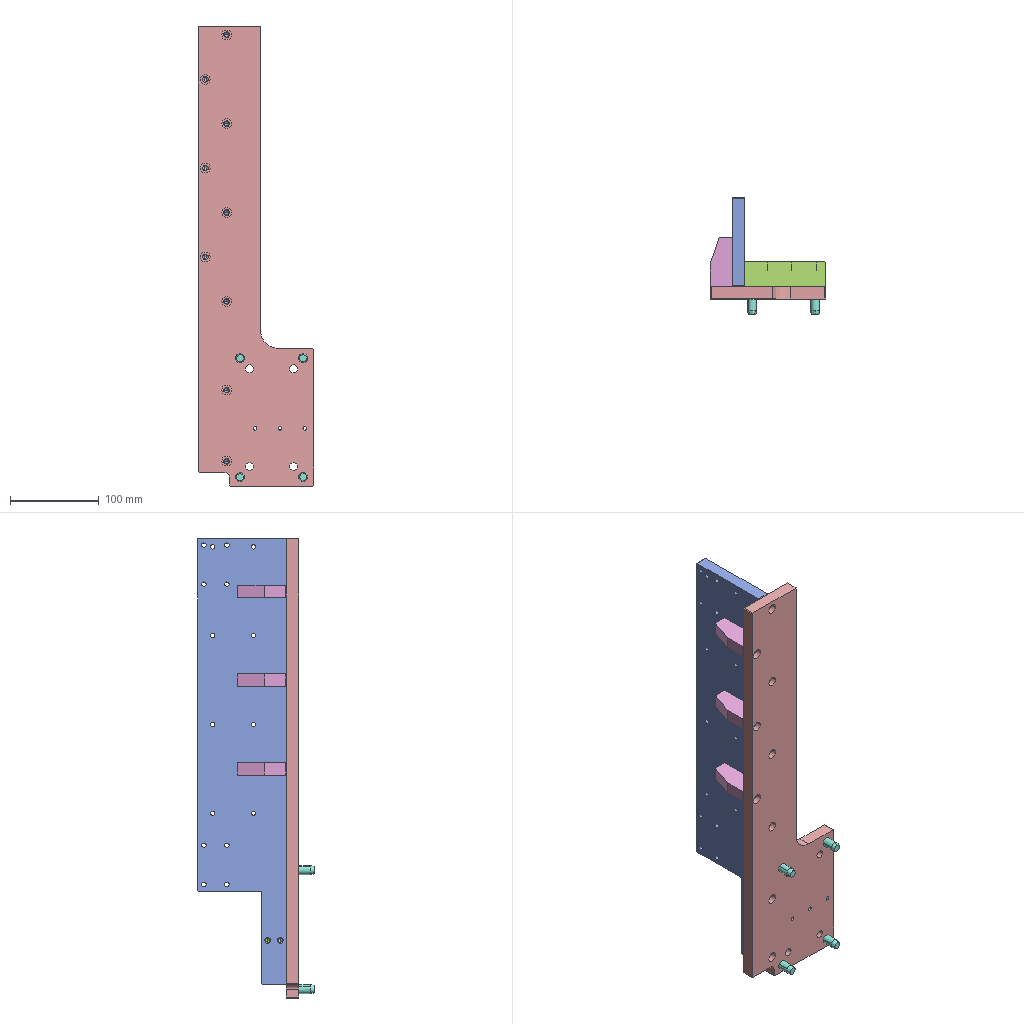Assembly | SolidWorks | 11 different items | 16 placed | box 130 x 132 x 518 mm
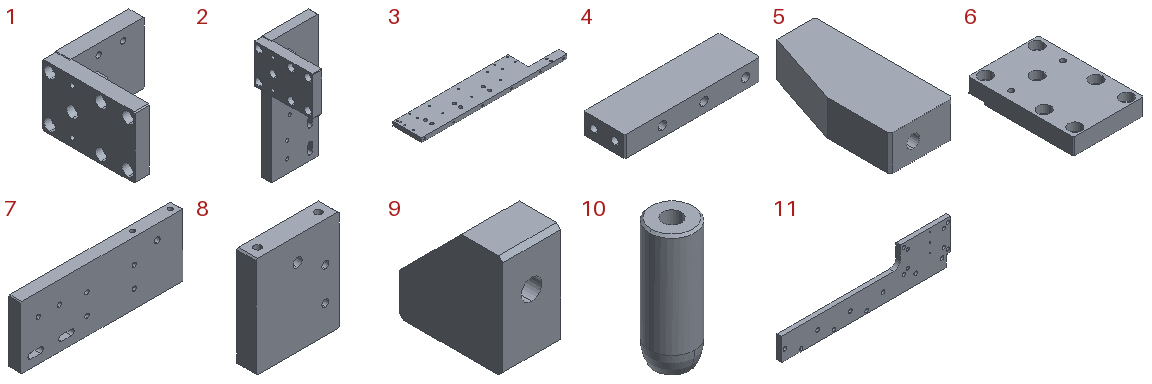Parts list (item | name | quantity | size | volume | features):
1 | (subassembly) | x1 | 85 x 90 x 60 mm | 133215 mm3 | -
2 | (subassembly) | x1 | 85 x 90 x 189 mm | 260889 mm3 | -
3 | - | x1 | 503 x 100 x 14 mm | 585787 mm3 | features HoleWzd 5, Chamfer 1, Extrusion 1, ICE 1
4 | - | x1 | 91 x 28 x 14 mm | 31396 mm3 | features HoleWzd 2, Chamfer 1, Extrusion 1
5 | - | x3 | 25 x 55 x 14 mm | 16216 mm3 | features HoleWzd 2, Chamfer 1, Extrusion 1
6 | - | x1 | 60 x 90 x 14 mm | 67395 mm3 | features HoleWzd 2, Chamfer 1, Extrusion 1, ICE 1
7 | - | x1 | 189 x 14 x 73 mm | 186915 mm3 | features HoleWzd 5, Chamfer 1, Extrusion 1
8 | - | x1 | 60 x 14 x 73 mm | 59241 mm3 | features HoleWzd 3, Chamfer 1, Extrusion 1
9 | - | x1 | 14 x 25 x 25 mm | 6579 mm3 | features HoleWzd 2, Chamfer 1, Extrusion 1
10 | - | x4 | 10 x 10 x 27.5 mm | 1957 mm3 | features BaseBody 1
11 | - | x1 | 518 x 14 x 130 mm | 616033 mm3 | features HoleWzd 5, ICE 3, Chamfer 2, Fillet 2, Extrusion 1
Mates (type | each side: item.copy, entity, surface, feature):
Coincident | 11.1 face plane Boss-Extrude1 | 3.1 face plane Boss-Extrude1
Coincident | 11.1 face plane Boss-Extrude1 | 4.1 face plane Boss-Extrude1
Concentric | 11.1 face cylinder M5 Tapped Hole1 | 4.1 face cylinder Hole Size per Socket Head Cap Screw Type1 | 2 times
Coincident | 11.1 face plane Boss-Extrude1 | 5.1 face plane Boss-Extrude2
Concentric | 3.1 face cylinder Hole Size per Socket Head Cap Screw Type1 | 5.1 face cylinder M6 Tapped Hole1 | 2 times
Coincident | 3.1 face plane Boss-Extrude1 | 5.1 face plane Boss-Extrude2
Concentric | 11.1 face cylinder Hole Size per Socket Head Cap Screw Type2 | 3.1 face cylinder M6 Tapped Hole3 | 2 times
Concentric | 11.1 face cylinder Cut-Extrude2 | 10.1 face cylinder Input1
Coincident | 11.1 face plane Cut-Extrude2 | 10.1 face plane Input1
Coincident | 11.1 face plane Cut-Extrude2 | 10.2 face plane Input1
Coincident | 11.1 face plane Cut-Extrude2 | 10.3 face plane Input1
Coincident | 11.1 face plane Cut-Extrude2 | 10.4 face plane Input1
Concentric | 11.1 face cylinder Cut-Extrude2 | 10.2 face cylinder Input1
Concentric | 11.1 face cylinder Cut-Extrude2 | 10.4 face cylinder Input1
Concentric | 11.1 face cylinder Cut-Extrude2 | 10.3 face cylinder Input1